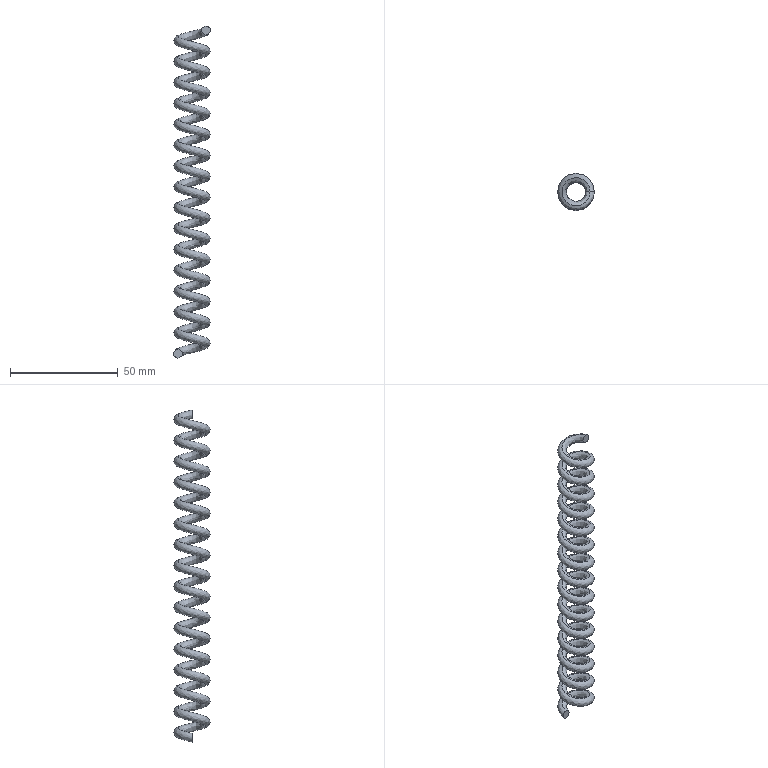Part | SolidWorks | features Helix 1, RefAxis 1, Sweep 1 | 1 solid | 4 faces | box 17 x 17 x 154 mm | volume 7958 mm3 | spline 2 | plane 2